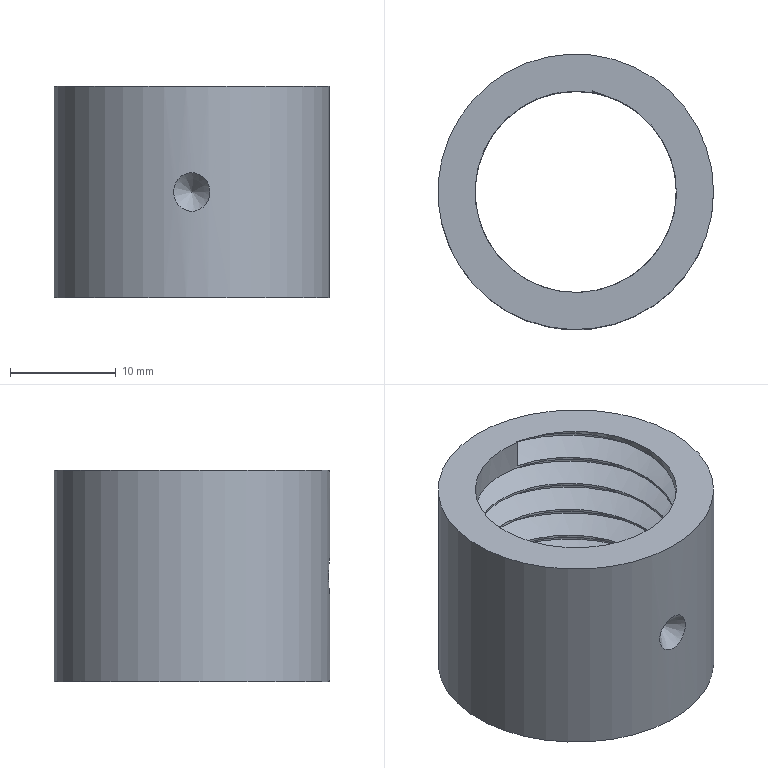Part | NX | features DATUM_CSYS 3, SKETCH 2, EXTRUDE 1, SWP104 1, THREADS 1 | 1 solid | 9 faces | box 26 x 26.176 x 20 mm | volume 3632 mm3 | cylinder 3 | plane 3 | spline 2 | cone 1 | commonest cylinder face diameters 19 x1 23 x1 26 x1